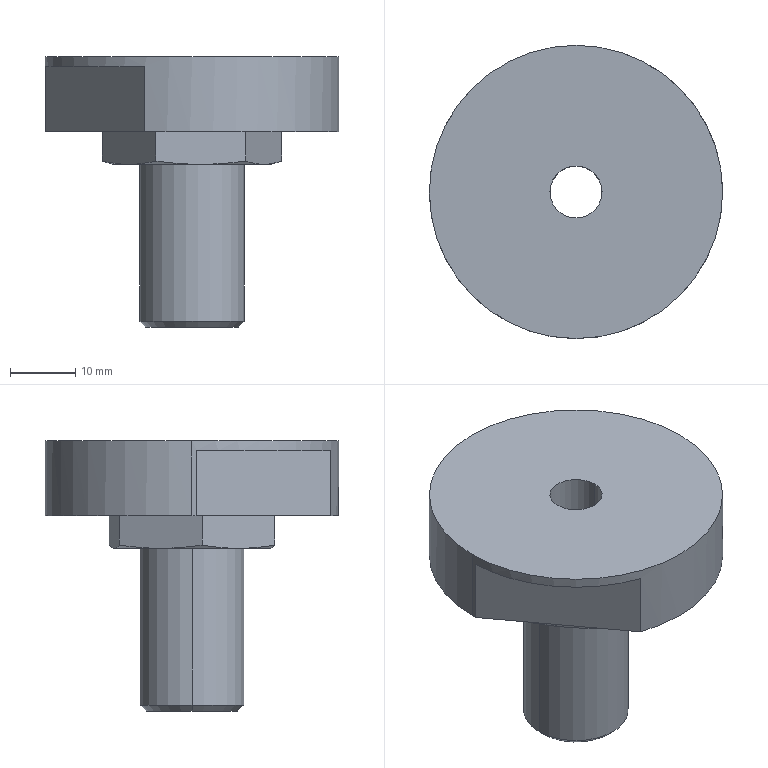Part | SolidWorks | features BaseBody 1 | 1 solid | 34 faces | box 45 x 45 x 41.5 mm | volume 22254 mm3 | plane 14 | cone 12 | cylinder 8 | commonest cylinder face diameters 8 x2 8.566 x2 16 x2 45 x2
STEP:
#1=CARTESIAN_POINT('',(-172.72,21.29,385.481));
#2=VERTEX_POINT('',#1);
#3=CARTESIAN_POINT('',(-202.5,0.,385.481));
#4=VERTEX_POINT('',#3);
#5=CARTESIAN_POINT('',(-180.,0.,385.481));
#6=DIRECTION('',(0.,0.,1.));
#7=DIRECTION('',(1.,0.,0.));
#8=AXIS2_PLACEMENT_3D('',#5,#6,#7);
#9=CIRCLE('',#8,22.5);
#10=EDGE_CURVE('',#2,#4,#9,.T.);
#11=ORIENTED_EDGE('',*,*,#10,.T.);
#12=CARTESIAN_POINT('',(-202.5,0.,396.981));
#13=VERTEX_POINT('',#12);
#14=CARTESIAN_POINT('',(-202.5,0.,391.231));
#15=DIRECTION('',(0.,0.,1.));
#16=VECTOR('',#15,1000.);
#17=LINE('',#14,#16);
#18=EDGE_CURVE('',#4,#13,#17,.T.);
#19=ORIENTED_EDGE('',*,*,#18,.T.);
#20=CARTESIAN_POINT('',(-157.5,0.,396.981));
#21=VERTEX_POINT('',#20);
#22=CARTESIAN_POINT('',(-180.,0.,396.981));
#23=DIRECTION('',(0.,0.,1.));
#24=DIRECTION('',(1.,0.,0.));
#25=AXIS2_PLACEMENT_3D('',#22,#23,#24);
#26=CIRCLE('',#25,22.5);
#27=EDGE_CURVE('',#21,#13,#26,.T.);
#28=ORIENTED_EDGE('',*,*,#27,.F.);
#29=CARTESIAN_POINT('',(-157.5,0.,385.481));
#30=VERTEX_POINT('',#29);
#31=CARTESIAN_POINT('',(-157.5,0.,391.231));
#32=DIRECTION('',(0.,0.,1.));
#33=VECTOR('',#32,1000.);
#34=LINE('',#31,#33);
#35=EDGE_CURVE('',#30,#21,#34,.T.);
#36=ORIENTED_EDGE('',*,*,#35,.F.);
#37=CARTESIAN_POINT('',(-157.51,0.6822,385.481));
#38=VERTEX_POINT('',#37);
#39=CARTESIAN_POINT('',(-180.,0.,385.481));
#40=DIRECTION('',(0.,0.,1.));
#41=DIRECTION('',(1.,0.,0.));
#42=AXIS2_PLACEMENT_3D('',#39,#40,#41);
#43=CIRCLE('',#42,22.5);
#44=EDGE_CURVE('',#30,#38,#43,.T.);
#45=ORIENTED_EDGE('',*,*,#44,.T.);
#46=CARTESIAN_POINT('',(-157.51,0.6822,395.481));
#47=VERTEX_POINT('',#46);
#48=CARTESIAN_POINT('',(-157.51,0.6822,391.231));
#49=DIRECTION('',(0.,0.,1.));
#50=VECTOR('',#49,1000.);
#51=LINE('',#48,#50);
#52=EDGE_CURVE('',#38,#47,#51,.T.);
#53=ORIENTED_EDGE('',*,*,#52,.T.);
#54=CARTESIAN_POINT('',(-172.72,21.29,395.481));
#55=VERTEX_POINT('',#54);
#56=CARTESIAN_POINT('',(-180.,0.,395.481));
#57=DIRECTION('',(0.,0.,1.));
#58=DIRECTION('',(1.,0.,0.));
#59=AXIS2_PLACEMENT_3D('',#56,#57,#58);
#60=CIRCLE('',#59,22.5);
#61=EDGE_CURVE('',#47,#55,#60,.T.);
#62=ORIENTED_EDGE('',*,*,#61,.T.);
#63=CARTESIAN_POINT('',(-172.72,21.29,391.231));
#64=DIRECTION('',(0.,0.,-1.));
#65=VECTOR('',#64,1000.);
#66=LINE('',#63,#65);
#67=EDGE_CURVE('',#55,#2,#66,.T.);
#68=ORIENTED_EDGE('',*,*,#67,.T.);
#69=EDGE_LOOP('',(#11,#19,#28,#36,#45,#53,#62,#68));
#70=FACE_OUTER_BOUND('',#69,.T.);
#71=CARTESIAN_POINT('',(-180.,0.,391.231));
#72=DIRECTION('',(0.,0.,1.));
#73=DIRECTION('',(1.,0.,0.));
#74=AXIS2_PLACEMENT_3D('',#71,#72,#73);
#75=CYLINDRICAL_SURFACE('',#74,22.5);
#76=ADVANCED_FACE('',(#70),#75,.T.);
#77=CARTESIAN_POINT('',(-184.,0.,361.844));
#78=VERTEX_POINT('',#77);
#79=CARTESIAN_POINT('',(-176.,0.,361.844));
#80=VERTEX_POINT('',#79);
#81=CARTESIAN_POINT('',(-180.,0.,361.844));
#82=DIRECTION('',(0.,0.,1.));
#83=DIRECTION('',(1.,0.,0.));
#84=AXIS2_PLACEMENT_3D('',#81,#82,#83);
#85=CIRCLE('',#84,4.);
#86=EDGE_CURVE('',#78,#80,#85,.T.);
#87=ORIENTED_EDGE('',*,*,#86,.F.);
#88=CARTESIAN_POINT('',(-184.,0.,396.981));
#89=VERTEX_POINT('',#88);
#90=CARTESIAN_POINT('',(-184.,0.,379.413));
#91=DIRECTION('',(0.,0.,1.));
#92=VECTOR('',#91,1000.);
#93=LINE('',#90,#92);
#94=EDGE_CURVE('',#78,#89,#93,.T.);
#95=ORIENTED_EDGE('',*,*,#94,.T.);
#96=CARTESIAN_POINT('',(-176.,0.,396.981));
#97=VERTEX_POINT('',#96);
#98=CARTESIAN_POINT('',(-180.,0.,396.981));
#99=DIRECTION('',(0.,0.,-1.));
#100=DIRECTION('',(1.,0.,0.));
#101=AXIS2_PLACEMENT_3D('',#98,#99,#100);
#102=CIRCLE('',#101,4.);
#103=EDGE_CURVE('',#97,#89,#102,.T.);
#104=ORIENTED_EDGE('',*,*,#103,.F.);
#105=CARTESIAN_POINT('',(-176.,0.,379.413));
#106=DIRECTION('',(0.,0.,1.));
#107=VECTOR('',#106,1000.);
#108=LINE('',#105,#107);
#109=EDGE_CURVE('',#80,#97,#108,.T.);
#110=ORIENTED_EDGE('',*,*,#109,.F.);
#111=EDGE_LOOP('',(#87,#95,#104,#110));
#112=FACE_OUTER_BOUND('',#111,.T.);
#113=CARTESIAN_POINT('',(-180.,0.,379.413));
#114=DIRECTION('',(0.,0.,1.));
#115=DIRECTION('',(1.,0.,0.));
#116=AXIS2_PLACEMENT_3D('',#113,#114,#115);
#117=CYLINDRICAL_SURFACE('',#116,4.);
#118=ADVANCED_FACE('',(#112),#117,.F.);
#119=ORIENTED_EDGE('',*,*,#86,.T.);
#120=CARTESIAN_POINT('',(-175.717,0.,361.681));
#121=VERTEX_POINT('',#120);
#122=CARTESIAN_POINT('',(-175.717,0.,361.681));
#123=DIRECTION('',(0.866,0.,-0.5));
#124=VECTOR('',#123,1000.);
#125=LINE('',#122,#124);
#126=EDGE_CURVE('',#80,#121,#125,.T.);
#127=ORIENTED_EDGE('',*,*,#126,.T.);
#128=CARTESIAN_POINT('',(-184.283,0.,361.681));
#129=VERTEX_POINT('',#128);
#130=CARTESIAN_POINT('',(-180.,0.,361.681));
#131=DIRECTION('',(0.,0.,1.));
#132=DIRECTION('',(-0.8046,-0.5938,0.));
#133=AXIS2_PLACEMENT_3D('',#130,#131,#132);
#134=CIRCLE('',#133,4.283);
#135=EDGE_CURVE('',#129,#121,#134,.T.);
#136=ORIENTED_EDGE('',*,*,#135,.F.);
#137=CARTESIAN_POINT('',(-184.283,0.,361.681));
#138=DIRECTION('',(-0.866,0.,-0.5));
#139=VECTOR('',#138,1000.);
#140=LINE('',#137,#139);
#141=EDGE_CURVE('',#78,#129,#140,.T.);
#142=ORIENTED_EDGE('',*,*,#141,.F.);
#143=EDGE_LOOP('',(#119,#127,#136,#142));
#144=FACE_OUTER_BOUND('',#143,.T.);
#145=CARTESIAN_POINT('',(-180.,0.,361.681));
#146=DIRECTION('',(0.,0.,-1.));
#147=DIRECTION('',(-1.,0.,0.));
#148=AXIS2_PLACEMENT_3D('',#145,#146,#147);
#149=CONICAL_SURFACE('',#148,4.283,1.047);
#150=ADVANCED_FACE('',(#144),#149,.F.);
#151=CARTESIAN_POINT('',(-184.283,0.,356.062));
#152=VERTEX_POINT('',#151);
#153=CARTESIAN_POINT('',(-175.717,0.,356.062));
#154=VERTEX_POINT('',#153);
#155=CARTESIAN_POINT('',(-180.,0.,356.062));
#156=DIRECTION('',(0.,0.,1.));
#157=DIRECTION('',(1.,0.,0.));
#158=AXIS2_PLACEMENT_3D('',#155,#156,#157);
#159=CIRCLE('',#158,4.283);
#160=EDGE_CURVE('',#152,#154,#159,.T.);
#161=ORIENTED_EDGE('',*,*,#160,.F.);
#162=CARTESIAN_POINT('',(-184.283,0.,358.872));
#163=DIRECTION('',(0.,0.,1.));
#164=VECTOR('',#163,1000.);
#165=LINE('',#162,#164);
#166=EDGE_CURVE('',#152,#129,#165,.T.);
#167=ORIENTED_EDGE('',*,*,#166,.T.);
#168=ORIENTED_EDGE('',*,*,#135,.T.);
#169=CARTESIAN_POINT('',(-175.717,0.,358.872));
#170=DIRECTION('',(0.,0.,1.));
#171=VECTOR('',#170,1000.);
#172=LINE('',#169,#171);
#173=EDGE_CURVE('',#154,#121,#172,.T.);
#174=ORIENTED_EDGE('',*,*,#173,.F.);
#175=EDGE_LOOP('',(#161,#167,#168,#174));
#176=FACE_OUTER_BOUND('',#175,.T.);
#177=CARTESIAN_POINT('',(-180.,0.,358.872));
#178=DIRECTION('',(0.,0.,1.));
#179=DIRECTION('',(1.,0.,0.));
#180=AXIS2_PLACEMENT_3D('',#177,#178,#179);
#181=CYLINDRICAL_SURFACE('',#180,4.283);
#182=ADVANCED_FACE('',(#176),#181,.F.);
#183=ORIENTED_EDGE('',*,*,#160,.T.);
#184=CARTESIAN_POINT('',(-175.136,0.,355.481));
#185=VERTEX_POINT('',#184);
#186=CARTESIAN_POINT('',(-175.136,0.,355.481));
#187=DIRECTION('',(0.7071,0.,-0.7071));
#188=VECTOR('',#187,1000.);
#189=LINE('',#186,#188);
#190=EDGE_CURVE('',#154,#185,#189,.T.);
#191=ORIENTED_EDGE('',*,*,#190,.T.);
#192=CARTESIAN_POINT('',(-184.864,0.,355.481));
#193=VERTEX_POINT('',#192);
#194=CARTESIAN_POINT('',(-180.,0.,355.481));
#195=DIRECTION('',(0.,0.,1.));
#196=DIRECTION('',(-1.,0.,0.));
#197=AXIS2_PLACEMENT_3D('',#194,#195,#196);
#198=CIRCLE('',#197,4.864);
#199=EDGE_CURVE('',#193,#185,#198,.T.);
#200=ORIENTED_EDGE('',*,*,#199,.F.);
#201=CARTESIAN_POINT('',(-184.864,0.,355.481));
#202=DIRECTION('',(-0.7071,0.,-0.7071));
#203=VECTOR('',#202,1000.);
#204=LINE('',#201,#203);
#205=EDGE_CURVE('',#152,#193,#204,.T.);
#206=ORIENTED_EDGE('',*,*,#205,.F.);
#207=EDGE_LOOP('',(#183,#191,#200,#206));
#208=FACE_OUTER_BOUND('',#207,.T.);
#209=CARTESIAN_POINT('',(-180.,0.,355.481));
#210=DIRECTION('',(0.,0.,-1.));
#211=DIRECTION('',(-1.,0.,0.));
#212=AXIS2_PLACEMENT_3D('',#209,#210,#211);
#213=CONICAL_SURFACE('',#212,4.864,0.7854);
#214=ADVANCED_FACE('',(#208),#213,.F.);
#215=CARTESIAN_POINT('',(-172.,0.,356.401));
#216=VERTEX_POINT('',#215);
#217=CARTESIAN_POINT('',(-188.,0.,356.401));
#218=VERTEX_POINT('',#217);
#219=CARTESIAN_POINT('',(-180.,0.,356.401));
#220=DIRECTION('',(0.,0.,1.));
#221=DIRECTION('',(1.,0.,0.));
#222=AXIS2_PLACEMENT_3D('',#219,#220,#221);
#223=CIRCLE('',#222,8.);
#224=EDGE_CURVE('',#216,#218,#223,.T.);
#225=ORIENTED_EDGE('',*,*,#224,.T.);
#226=CARTESIAN_POINT('',(-188.,0.,380.481));
#227=VERTEX_POINT('',#226);
#228=CARTESIAN_POINT('',(-188.,0.,368.441));
#229=DIRECTION('',(0.,0.,1.));
#230=VECTOR('',#229,1000.);
#231=LINE('',#228,#230);
#232=EDGE_CURVE('',#218,#227,#231,.T.);
#233=ORIENTED_EDGE('',*,*,#232,.T.);
#234=CARTESIAN_POINT('',(-172.,0.,380.481));
#235=VERTEX_POINT('',#234);
#236=CARTESIAN_POINT('',(-180.,0.,380.481));
#237=DIRECTION('',(0.,0.,1.));
#238=DIRECTION('',(1.,0.,0.));
#239=AXIS2_PLACEMENT_3D('',#236,#237,#238);
#240=CIRCLE('',#239,8.);
#241=EDGE_CURVE('',#235,#227,#240,.T.);
#242=ORIENTED_EDGE('',*,*,#241,.F.);
#243=CARTESIAN_POINT('',(-172.,0.,368.441));
#244=DIRECTION('',(0.,0.,1.));
#245=VECTOR('',#244,1000.);
#246=LINE('',#243,#245);
#247=EDGE_CURVE('',#216,#235,#246,.T.);
#248=ORIENTED_EDGE('',*,*,#247,.F.);
#249=EDGE_LOOP('',(#225,#233,#242,#248));
#250=FACE_OUTER_BOUND('',#249,.T.);
#251=CARTESIAN_POINT('',(-180.,0.,368.441));
#252=DIRECTION('',(0.,0.,1.));
#253=DIRECTION('',(1.,0.,0.));
#254=AXIS2_PLACEMENT_3D('',#251,#252,#253);
#255=CYLINDRICAL_SURFACE('',#254,8.);
#256=ADVANCED_FACE('',(#250),#255,.T.);
#257=CARTESIAN_POINT('',(-187.08,0.,355.481));
#258=VERTEX_POINT('',#257);
#259=CARTESIAN_POINT('',(-172.92,0.,355.481));
#260=VERTEX_POINT('',#259);
#261=CARTESIAN_POINT('',(-180.,0.,355.481));
#262=DIRECTION('',(0.,0.,-1.));
#263=DIRECTION('',(1.,0.,0.));
#264=AXIS2_PLACEMENT_3D('',#261,#262,#263);
#265=CIRCLE('',#264,7.08);
#266=EDGE_CURVE('',#258,#260,#265,.T.);
#267=ORIENTED_EDGE('',*,*,#266,.F.);
#268=CARTESIAN_POINT('',(-188.,0.,356.401));
#269=DIRECTION('',(-0.7071,0.,0.7071));
#270=VECTOR('',#269,1000.);
#271=LINE('',#268,#270);
#272=EDGE_CURVE('',#258,#218,#271,.T.);
#273=ORIENTED_EDGE('',*,*,#272,.T.);
#274=ORIENTED_EDGE('',*,*,#224,.F.);
#275=CARTESIAN_POINT('',(-172.,0.,356.401));
#276=DIRECTION('',(0.7071,0.,0.7071));
#277=VECTOR('',#276,1000.);
#278=LINE('',#275,#277);
#279=EDGE_CURVE('',#260,#216,#278,.T.);
#280=ORIENTED_EDGE('',*,*,#279,.F.);
#281=EDGE_LOOP('',(#267,#273,#274,#280));
#282=FACE_OUTER_BOUND('',#281,.T.);
#283=CARTESIAN_POINT('',(-180.,0.,356.401));
#284=DIRECTION('',(0.,0.,1.));
#285=DIRECTION('',(1.,0.,0.));
#286=AXIS2_PLACEMENT_3D('',#283,#284,#285);
#287=CONICAL_SURFACE('',#286,8.,0.7854);
#288=ADVANCED_FACE('',(#282),#287,.T.);
#289=ORIENTED_EDGE('',*,*,#27,.T.);
#290=CARTESIAN_POINT('',(-180.,0.,396.981));
#291=DIRECTION('',(0.,0.,1.));
#292=DIRECTION('',(1.,0.,0.));
#293=AXIS2_PLACEMENT_3D('',#290,#291,#292);
#294=CIRCLE('',#293,22.5);
#295=EDGE_CURVE('',#13,#21,#294,.T.);
#296=ORIENTED_EDGE('',*,*,#295,.T.);
#297=EDGE_LOOP('',(#289,#296));
#298=FACE_OUTER_BOUND('',#297,.T.);
#299=ORIENTED_EDGE('',*,*,#103,.T.);
#300=CARTESIAN_POINT('',(-180.,0.,396.981));
#301=DIRECTION('',(0.,0.,-1.));
#302=DIRECTION('',(1.,0.,0.));
#303=AXIS2_PLACEMENT_3D('',#300,#301,#302);
#304=CIRCLE('',#303,4.);
#305=EDGE_CURVE('',#89,#97,#304,.T.);
#306=ORIENTED_EDGE('',*,*,#305,.T.);
#307=EDGE_LOOP('',(#299,#306));
#308=FACE_BOUND('',#307,.T.);
#309=CARTESIAN_POINT('',(-187.868,10.661,396.981));
#310=DIRECTION('',(0.,0.,1.));
#311=DIRECTION('',(1.,0.,0.));
#312=AXIS2_PLACEMENT_3D('',#309,#310,#311);
#313=PLANE('',#312);
#314=ADVANCED_FACE('',(#298,#308),#313,.T.);
#315=ORIENTED_EDGE('',*,*,#18,.F.);
#316=CARTESIAN_POINT('',(-202.49,-0.6822,385.481));
#317=VERTEX_POINT('',#316);
#318=CARTESIAN_POINT('',(-180.,0.,385.481));
#319=DIRECTION('',(0.,0.,1.));
#320=DIRECTION('',(1.,0.,0.));
#321=AXIS2_PLACEMENT_3D('',#318,#319,#320);
#322=CIRCLE('',#321,22.5);
#323=EDGE_CURVE('',#4,#317,#322,.T.);
#324=ORIENTED_EDGE('',*,*,#323,.T.);
#325=CARTESIAN_POINT('',(-202.49,-0.6822,395.481));
#326=VERTEX_POINT('',#325);
#327=CARTESIAN_POINT('',(-202.49,-0.6822,391.231));
#328=DIRECTION('',(0.,0.,1.));
#329=VECTOR('',#328,1000.);
#330=LINE('',#327,#329);
#331=EDGE_CURVE('',#317,#326,#330,.T.);
#332=ORIENTED_EDGE('',*,*,#331,.T.);
#333=CARTESIAN_POINT('',(-187.28,-21.29,395.481));
#334=VERTEX_POINT('',#333);
#335=CARTESIAN_POINT('',(-180.,0.,395.481));
#336=DIRECTION('',(0.,0.,1.));
#337=DIRECTION('',(1.,0.,0.));
#338=AXIS2_PLACEMENT_3D('',#335,#336,#337);
#339=CIRCLE('',#338,22.5);
#340=EDGE_CURVE('',#326,#334,#339,.T.);
#341=ORIENTED_EDGE('',*,*,#340,.T.);
#342=CARTESIAN_POINT('',(-187.28,-21.29,385.481));
#343=VERTEX_POINT('',#342);
#344=CARTESIAN_POINT('',(-187.28,-21.29,391.231));
#345=DIRECTION('',(0.,0.,-1.));
#346=VECTOR('',#345,1000.);
#347=LINE('',#344,#346);
#348=EDGE_CURVE('',#334,#343,#347,.T.);
#349=ORIENTED_EDGE('',*,*,#348,.T.);
#350=CARTESIAN_POINT('',(-180.,0.,385.481));
#351=DIRECTION('',(0.,0.,1.));
#352=DIRECTION('',(1.,0.,0.));
#353=AXIS2_PLACEMENT_3D('',#350,#351,#352);
#354=CIRCLE('',#353,22.5);
#355=EDGE_CURVE('',#343,#30,#354,.T.);
#356=ORIENTED_EDGE('',*,*,#355,.T.);
#357=ORIENTED_EDGE('',*,*,#35,.T.);
#358=ORIENTED_EDGE('',*,*,#295,.F.);
#359=EDGE_LOOP('',(#315,#324,#332,#341,#349,#356,#357,#358));
#360=FACE_OUTER_BOUND('',#359,.T.);
#361=CARTESIAN_POINT('',(-180.,0.,391.231));
#362=DIRECTION('',(0.,0.,1.));
#363=DIRECTION('',(1.,0.,0.));
#364=AXIS2_PLACEMENT_3D('',#361,#362,#363);
#365=CYLINDRICAL_SURFACE('',#364,22.5);
#366=ADVANCED_FACE('',(#360),#365,.T.);
#367=ORIENTED_EDGE('',*,*,#94,.F.);
#368=CARTESIAN_POINT('',(-180.,0.,361.844));
#369=DIRECTION('',(0.,0.,1.));
#370=DIRECTION('',(1.,0.,0.));
#371=AXIS2_PLACEMENT_3D('',#368,#369,#370);
#372=CIRCLE('',#371,4.);
#373=EDGE_CURVE('',#80,#78,#372,.T.);
#374=ORIENTED_EDGE('',*,*,#373,.F.);
#375=ORIENTED_EDGE('',*,*,#109,.T.);
#376=ORIENTED_EDGE('',*,*,#305,.F.);
#377=EDGE_LOOP('',(#367,#374,#375,#376));
#378=FACE_OUTER_BOUND('',#377,.T.);
#379=CARTESIAN_POINT('',(-180.,0.,379.413));
#380=DIRECTION('',(0.,0.,1.));
#381=DIRECTION('',(1.,0.,0.));
#382=AXIS2_PLACEMENT_3D('',#379,#380,#381);
#383=CYLINDRICAL_SURFACE('',#382,4.);
#384=ADVANCED_FACE('',(#378),#383,.F.);
#385=CARTESIAN_POINT('',(-187.28,-21.29,385.481));
#386=DIRECTION('',(-0.5938,0.8046,0.));
#387=VECTOR('',#386,1000.);
#388=LINE('',#385,#387);
#389=EDGE_CURVE('',#343,#317,#388,.T.);
#390=ORIENTED_EDGE('',*,*,#389,.T.);
#391=ORIENTED_EDGE('',*,*,#323,.F.);
#392=ORIENTED_EDGE('',*,*,#10,.F.);
#393=CARTESIAN_POINT('',(-172.72,21.29,385.481));
#394=DIRECTION('',(0.5938,-0.8046,0.));
#395=VECTOR('',#394,1000.);
#396=LINE('',#393,#395);
#397=EDGE_CURVE('',#2,#38,#396,.T.);
#398=ORIENTED_EDGE('',*,*,#397,.T.);
#399=ORIENTED_EDGE('',*,*,#44,.F.);
#400=ORIENTED_EDGE('',*,*,#355,.F.);
#401=EDGE_LOOP('',(#390,#391,#392,#398,#399,#400));
#402=FACE_OUTER_BOUND('',#401,.T.);
#403=CARTESIAN_POINT('',(-174.459,12.7,385.481));
#404=VERTEX_POINT('',#403);
#405=CARTESIAN_POINT('',(-188.228,11.149,385.481));
#406=VERTEX_POINT('',#405);
#407=CARTESIAN_POINT('',(-174.459,12.7,385.481));
#408=DIRECTION('',(-0.9937,-0.112,0.));
#409=VECTOR('',#408,1000.);
#410=LINE('',#407,#409);
#411=EDGE_CURVE('',#404,#406,#410,.T.);
#412=ORIENTED_EDGE('',*,*,#411,.T.);
#413=CARTESIAN_POINT('',(-193.769,-1.552,385.481));
#414=VERTEX_POINT('',#413);
#415=CARTESIAN_POINT('',(-188.228,11.149,385.481));
#416=DIRECTION('',(-0.3999,-0.9166,0.));
#417=VECTOR('',#416,1000.);
#418=LINE('',#415,#417);
#419=EDGE_CURVE('',#406,#414,#418,.T.);
#420=ORIENTED_EDGE('',*,*,#419,.T.);
#421=CARTESIAN_POINT('',(-185.541,-12.7,385.481));
#422=VERTEX_POINT('',#421);
#423=CARTESIAN_POINT('',(-193.769,-1.552,385.481));
#424=DIRECTION('',(0.5938,-0.8046,0.));
#425=VECTOR('',#424,1000.);
#426=LINE('',#423,#425);
#427=EDGE_CURVE('',#414,#422,#426,.T.);
#428=ORIENTED_EDGE('',*,*,#427,.T.);
#429=CARTESIAN_POINT('',(-171.772,-11.149,385.481));
#430=VERTEX_POINT('',#429);
#431=CARTESIAN_POINT('',(-185.541,-12.7,385.481));
#432=DIRECTION('',(0.9937,0.112,0.));
#433=VECTOR('',#432,1000.);
#434=LINE('',#431,#433);
#435=EDGE_CURVE('',#422,#430,#434,.T.);
#436=ORIENTED_EDGE('',*,*,#435,.T.);
#437=CARTESIAN_POINT('',(-166.231,1.552,385.481));
#438=VERTEX_POINT('',#437);
#439=CARTESIAN_POINT('',(-171.772,-11.149,385.481));
#440=DIRECTION('',(0.3999,0.9166,0.));
#441=VECTOR('',#440,1000.);
#442=LINE('',#439,#441);
#443=EDGE_CURVE('',#430,#438,#442,.T.);
#444=ORIENTED_EDGE('',*,*,#443,.T.);
#445=CARTESIAN_POINT('',(-166.231,1.552,385.481));
#446=DIRECTION('',(-0.5938,0.8046,0.));
#447=VECTOR('',#446,1000.);
#448=LINE('',#445,#447);
#449=EDGE_CURVE('',#438,#404,#448,.T.);
#450=ORIENTED_EDGE('',*,*,#449,.T.);
#451=EDGE_LOOP('',(#412,#420,#428,#436,#444,#450));
#452=FACE_BOUND('',#451,.T.);
#453=CARTESIAN_POINT('',(-192.381,16.776,385.481));
#454=DIRECTION('',(0.,0.,-1.));
#455=DIRECTION('',(-1.,0.,0.));
#456=AXIS2_PLACEMENT_3D('',#453,#454,#455);
#457=PLANE('',#456);
#458=ADVANCED_FACE('',(#402,#452),#457,.T.);
#459=ORIENTED_EDGE('',*,*,#67,.F.);
#460=CARTESIAN_POINT('',(-188.869,43.169,395.481));
#461=DIRECTION('',(-0.5938,0.8046,0.));
#462=VECTOR('',#461,1000.);
#463=LINE('',#460,#462);
#464=EDGE_CURVE('',#47,#55,#463,.T.);
#465=ORIENTED_EDGE('',*,*,#464,.F.);
#466=ORIENTED_EDGE('',*,*,#52,.F.);
#467=ORIENTED_EDGE('',*,*,#397,.F.);
#468=EDGE_LOOP('',(#459,#465,#466,#467));
#469=FACE_OUTER_BOUND('',#468,.T.);
#470=CARTESIAN_POINT('',(-188.869,43.169,395.481));
#471=DIRECTION('',(-0.8046,-0.5938,0.));
#472=DIRECTION('',(0.5938,-0.8046,0.));
#473=AXIS2_PLACEMENT_3D('',#470,#471,#472);
#474=PLANE('',#473);
#475=ADVANCED_FACE('',(#469),#474,.F.);
#476=ORIENTED_EDGE('',*,*,#61,.F.);
#477=ORIENTED_EDGE('',*,*,#464,.T.);
#478=EDGE_LOOP('',(#476,#477));
#479=FACE_OUTER_BOUND('',#478,.T.);
#480=CARTESIAN_POINT('',(-180.,0.,395.481));
#481=DIRECTION('',(0.,0.,-1.));
#482=DIRECTION('',(-1.,0.,0.));
#483=AXIS2_PLACEMENT_3D('',#480,#481,#482);
#484=PLANE('',#483);
#485=ADVANCED_FACE('',(#479),#484,.T.);
#486=ORIENTED_EDGE('',*,*,#348,.F.);
#487=CARTESIAN_POINT('',(-171.131,-43.169,395.481));
#488=DIRECTION('',(0.5938,-0.8046,0.));
#489=VECTOR('',#488,1000.);
#490=LINE('',#487,#489);
#491=EDGE_CURVE('',#326,#334,#490,.T.);
#492=ORIENTED_EDGE('',*,*,#491,.F.);
#493=ORIENTED_EDGE('',*,*,#331,.F.);
#494=ORIENTED_EDGE('',*,*,#389,.F.);
#495=EDGE_LOOP('',(#486,#492,#493,#494));
#496=FACE_OUTER_BOUND('',#495,.T.);
#497=CARTESIAN_POINT('',(-171.131,-43.169,395.481));
#498=DIRECTION('',(0.8046,0.5938,0.));
#499=DIRECTION('',(-0.5938,0.8046,0.));
#500=AXIS2_PLACEMENT_3D('',#497,#498,#499);
#501=PLANE('',#500);
#502=ADVANCED_FACE('',(#496),#501,.F.);
#503=ORIENTED_EDGE('',*,*,#340,.F.);
#504=ORIENTED_EDGE('',*,*,#491,.T.);
#505=EDGE_LOOP('',(#503,#504));
#506=FACE_OUTER_BOUND('',#505,.T.);
#507=CARTESIAN_POINT('',(-180.,0.,395.481));
#508=DIRECTION('',(0.,0.,-1.));
#509=DIRECTION('',(-1.,0.,0.));
#510=AXIS2_PLACEMENT_3D('',#507,#508,#509);
#511=PLANE('',#510);
#512=ADVANCED_FACE('',(#506),#511,.T.);
#513=ORIENTED_EDGE('',*,*,#126,.F.);
#514=ORIENTED_EDGE('',*,*,#373,.T.);
#515=ORIENTED_EDGE('',*,*,#141,.T.);
#516=CARTESIAN_POINT('',(-180.,0.,361.681));
#517=DIRECTION('',(0.,0.,1.));
#518=DIRECTION('',(-0.8046,-0.5938,0.));
#519=AXIS2_PLACEMENT_3D('',#516,#517,#518);
#520=CIRCLE('',#519,4.283);
#521=EDGE_CURVE('',#121,#129,#520,.T.);
#522=ORIENTED_EDGE('',*,*,#521,.F.);
#523=EDGE_LOOP('',(#513,#514,#515,#522));
#524=FACE_OUTER_BOUND('',#523,.T.);
#525=CARTESIAN_POINT('',(-180.,0.,361.681));
#526=DIRECTION('',(0.,0.,-1.));
#527=DIRECTION('',(-1.,0.,0.));
#528=AXIS2_PLACEMENT_3D('',#525,#526,#527);
#529=CONICAL_SURFACE('',#528,4.283,1.047);
#530=ADVANCED_FACE('',(#524),#529,.F.);
#531=CARTESIAN_POINT('',(-193.769,-1.552,380.978));
#532=VERTEX_POINT('',#531);
#533=CARTESIAN_POINT('',(-193.769,-1.552,385.481));
#534=DIRECTION('',(0.,0.,-1.));
#535=VECTOR('',#534,1000.);
#536=LINE('',#533,#535);
#537=EDGE_CURVE('',#414,#532,#536,.T.);
#538=ORIENTED_EDGE('',*,*,#537,.F.);
#539=ORIENTED_EDGE('',*,*,#419,.F.);
#540=CARTESIAN_POINT('',(-188.228,11.149,380.978));
#541=VERTEX_POINT('',#540);
#542=CARTESIAN_POINT('',(-188.228,11.149,385.481));
#543=DIRECTION('',(0.,0.,1.));
#544=VECTOR('',#543,1000.);
#545=LINE('',#542,#544);
#546=EDGE_CURVE('',#541,#406,#545,.T.);
#547=ORIENTED_EDGE('',*,*,#546,.F.);
#548=CARTESIAN_POINT('',(-190.999,4.798,380.481));
#549=VERTEX_POINT('',#548);
#550=CARTESIAN_POINT('',(-190.999,4.798,380.481));
#551=CARTESIAN_POINT('',(-190.535,5.862,380.481));
#552=CARTESIAN_POINT('',(-190.072,6.923,380.527));
#553=CARTESIAN_POINT('',(-189.149,9.039,380.699));
#554=CARTESIAN_POINT('',(-188.688,10.095,380.824));
#555=CARTESIAN_POINT('',(-188.228,11.149,380.978));
#556=B_SPLINE_CURVE_WITH_KNOTS('',3,(#550,#551,#552,#553,#554,#555),.UNSPECIFIED.,.F.,.F.,(4,2,4),(0.,0.003473,0.006946),.UNSPECIFIED.);
#557=EDGE_CURVE('',#549,#541,#556,.T.);
#558=ORIENTED_EDGE('',*,*,#557,.F.);
#559=CARTESIAN_POINT('',(-193.769,-1.552,380.978));
#560=CARTESIAN_POINT('',(-193.31,-0.498,380.824));
#561=CARTESIAN_POINT('',(-192.849,0.5576,380.699));
#562=CARTESIAN_POINT('',(-191.926,2.674,380.527));
#563=CARTESIAN_POINT('',(-191.463,3.735,380.481));
#564=CARTESIAN_POINT('',(-190.999,4.798,380.481));
#565=B_SPLINE_CURVE_WITH_KNOTS('',3,(#559,#560,#561,#562,#563,#564),.UNSPECIFIED.,.F.,.F.,(4,2,4),(0.,0.003473,0.006946),.UNSPECIFIED.);
#566=EDGE_CURVE('',#532,#549,#565,.T.);
#567=ORIENTED_EDGE('',*,*,#566,.F.);
#568=EDGE_LOOP('',(#538,#539,#547,#558,#567));
#569=FACE_OUTER_BOUND('',#568,.T.);
#570=CARTESIAN_POINT('',(-193.769,-1.552,385.481));
#571=DIRECTION('',(0.9166,-0.3999,0.));
#572=DIRECTION('',(0.3999,0.9166,0.));
#573=AXIS2_PLACEMENT_3D('',#570,#571,#572);
#574=PLANE('',#573);
#575=ADVANCED_FACE('',(#569),#574,.F.);
#576=ORIENTED_EDGE('',*,*,#411,.F.);
#577=CARTESIAN_POINT('',(-174.459,12.7,380.978));
#578=VERTEX_POINT('',#577);
#579=CARTESIAN_POINT('',(-174.459,12.7,385.481));
#580=DIRECTION('',(0.,0.,1.));
#581=VECTOR('',#580,1000.);
#582=LINE('',#579,#581);
#583=EDGE_CURVE('',#578,#404,#582,.T.);
#584=ORIENTED_EDGE('',*,*,#583,.F.);
#585=CARTESIAN_POINT('',(-181.344,11.925,380.481));
#586=VERTEX_POINT('',#585);
#587=CARTESIAN_POINT('',(-181.344,11.925,380.481));
#588=CARTESIAN_POINT('',(-180.19,12.054,380.481));
#589=CARTESIAN_POINT('',(-179.04,12.184,380.527));
#590=CARTESIAN_POINT('',(-176.746,12.443,380.699));
#591=CARTESIAN_POINT('',(-175.602,12.572,380.824));
#592=CARTESIAN_POINT('',(-174.459,12.7,380.978));
#593=B_SPLINE_CURVE_WITH_KNOTS('',3,(#587,#588,#589,#590,#591,#592),.UNSPECIFIED.,.F.,.F.,(4,2,4),(0.,0.003473,0.006946),.UNSPECIFIED.);
#594=EDGE_CURVE('',#586,#578,#593,.T.);
#595=ORIENTED_EDGE('',*,*,#594,.F.);
#596=CARTESIAN_POINT('',(-188.228,11.149,380.978));
#597=CARTESIAN_POINT('',(-187.086,11.277,380.824));
#598=CARTESIAN_POINT('',(-185.942,11.406,380.699));
#599=CARTESIAN_POINT('',(-183.647,11.665,380.527));
#600=CARTESIAN_POINT('',(-182.497,11.795,380.481));
#601=CARTESIAN_POINT('',(-181.344,11.925,380.481));
#602=B_SPLINE_CURVE_WITH_KNOTS('',3,(#596,#597,#598,#599,#600,#601),.UNSPECIFIED.,.F.,.F.,(4,2,4),(0.,0.003473,0.006946),.UNSPECIFIED.);
#603=EDGE_CURVE('',#541,#586,#602,.T.);
#604=ORIENTED_EDGE('',*,*,#603,.F.);
#605=ORIENTED_EDGE('',*,*,#546,.T.);
#606=EDGE_LOOP('',(#576,#584,#595,#604,#605));
#607=FACE_OUTER_BOUND('',#606,.T.);
#608=CARTESIAN_POINT('',(-188.228,11.149,385.481));
#609=DIRECTION('',(0.112,-0.9937,0.));
#610=DIRECTION('',(0.9937,0.112,0.));
#611=AXIS2_PLACEMENT_3D('',#608,#609,#610);
#612=PLANE('',#611);
#613=ADVANCED_FACE('',(#607),#612,.F.);
#614=ORIENTED_EDGE('',*,*,#449,.F.);
#615=CARTESIAN_POINT('',(-166.231,1.552,380.978));
#616=VERTEX_POINT('',#615);
#617=CARTESIAN_POINT('',(-166.231,1.552,385.481));
#618=DIRECTION('',(0.,0.,1.));
#619=VECTOR('',#618,1000.);
#620=LINE('',#617,#619);
#621=EDGE_CURVE('',#616,#438,#620,.T.);
#622=ORIENTED_EDGE('',*,*,#621,.F.);
#623=CARTESIAN_POINT('',(-170.345,7.126,380.481));
#624=VERTEX_POINT('',#623);
#625=CARTESIAN_POINT('',(-170.345,7.126,380.481));
#626=CARTESIAN_POINT('',(-169.656,6.192,380.481));
#627=CARTESIAN_POINT('',(-168.968,5.261,380.527));
#628=CARTESIAN_POINT('',(-167.597,3.403,380.699));
#629=CARTESIAN_POINT('',(-166.913,2.477,380.824));
#630=CARTESIAN_POINT('',(-166.231,1.552,380.978));
#631=B_SPLINE_CURVE_WITH_KNOTS('',3,(#625,#626,#627,#628,#629,#630),.UNSPECIFIED.,.F.,.F.,(4,2,4),(0.,0.003473,0.006946),.UNSPECIFIED.);
#632=EDGE_CURVE('',#624,#616,#631,.T.);
#633=ORIENTED_EDGE('',*,*,#632,.F.);
#634=CARTESIAN_POINT('',(-174.459,12.7,380.978));
#635=CARTESIAN_POINT('',(-173.777,11.775,380.824));
#636=CARTESIAN_POINT('',(-173.093,10.849,380.699));
#637=CARTESIAN_POINT('',(-171.721,8.991,380.527));
#638=CARTESIAN_POINT('',(-171.034,8.06,380.481));
#639=CARTESIAN_POINT('',(-170.345,7.126,380.481));
#640=B_SPLINE_CURVE_WITH_KNOTS('',3,(#634,#635,#636,#637,#638,#639),.UNSPECIFIED.,.F.,.F.,(4,2,4),(0.,0.003473,0.006946),.UNSPECIFIED.);
#641=EDGE_CURVE('',#578,#624,#640,.T.);
#642=ORIENTED_EDGE('',*,*,#641,.F.);
#643=ORIENTED_EDGE('',*,*,#583,.T.);
#644=EDGE_LOOP('',(#614,#622,#633,#642,#643));
#645=FACE_OUTER_BOUND('',#644,.T.);
#646=CARTESIAN_POINT('',(-174.459,12.7,385.481));
#647=DIRECTION('',(-0.8046,-0.5938,0.));
#648=DIRECTION('',(0.5938,-0.8046,0.));
#649=AXIS2_PLACEMENT_3D('',#646,#647,#648);
#650=PLANE('',#649);
#651=ADVANCED_FACE('',(#645),#650,.F.);
#652=ORIENTED_EDGE('',*,*,#443,.F.);
#653=CARTESIAN_POINT('',(-171.772,-11.149,380.978));
#654=VERTEX_POINT('',#653);
#655=CARTESIAN_POINT('',(-171.772,-11.149,385.481));
#656=DIRECTION('',(0.,0.,1.));
#657=VECTOR('',#656,1000.);
#658=LINE('',#655,#657);
#659=EDGE_CURVE('',#654,#430,#658,.T.);
#660=ORIENTED_EDGE('',*,*,#659,.F.);
#661=CARTESIAN_POINT('',(-169.001,-4.798,380.481));
#662=VERTEX_POINT('',#661);
#663=CARTESIAN_POINT('',(-169.001,-4.798,380.481));
#664=CARTESIAN_POINT('',(-169.465,-5.862,380.481));
#665=CARTESIAN_POINT('',(-169.928,-6.923,380.527));
#666=CARTESIAN_POINT('',(-170.851,-9.039,380.699));
#667=CARTESIAN_POINT('',(-171.312,-10.095,380.824));
#668=CARTESIAN_POINT('',(-171.772,-11.149,380.978));
#669=B_SPLINE_CURVE_WITH_KNOTS('',3,(#663,#664,#665,#666,#667,#668),.UNSPECIFIED.,.F.,.F.,(4,2,4),(0.,0.003473,0.006946),.UNSPECIFIED.);
#670=EDGE_CURVE('',#662,#654,#669,.T.);
#671=ORIENTED_EDGE('',*,*,#670,.F.);
#672=CARTESIAN_POINT('',(-166.231,1.552,380.978));
#673=CARTESIAN_POINT('',(-166.69,0.498,380.824));
#674=CARTESIAN_POINT('',(-167.151,-0.5576,380.699));
#675=CARTESIAN_POINT('',(-168.074,-2.674,380.527));
#676=CARTESIAN_POINT('',(-168.537,-3.735,380.481));
#677=CARTESIAN_POINT('',(-169.001,-4.798,380.481));
#678=B_SPLINE_CURVE_WITH_KNOTS('',3,(#672,#673,#674,#675,#676,#677),.UNSPECIFIED.,.F.,.F.,(4,2,4),(0.,0.003473,0.006946),.UNSPECIFIED.);
#679=EDGE_CURVE('',#616,#662,#678,.T.);
#680=ORIENTED_EDGE('',*,*,#679,.F.);
#681=ORIENTED_EDGE('',*,*,#621,.T.);
#682=EDGE_LOOP('',(#652,#660,#671,#680,#681));
#683=FACE_OUTER_BOUND('',#682,.T.);
#684=CARTESIAN_POINT('',(-166.231,1.552,385.481));
#685=DIRECTION('',(-0.9166,0.3999,0.));
#686=DIRECTION('',(-0.3999,-0.9166,0.));
#687=AXIS2_PLACEMENT_3D('',#684,#685,#686);
#688=PLANE('',#687);
#689=ADVANCED_FACE('',(#683),#688,.F.);
#690=ORIENTED_EDGE('',*,*,#659,.T.);
#691=ORIENTED_EDGE('',*,*,#435,.F.);
#692=CARTESIAN_POINT('',(-185.541,-12.7,380.978));
#693=VERTEX_POINT('',#692);
#694=CARTESIAN_POINT('',(-185.541,-12.7,385.481));
#695=DIRECTION('',(0.,0.,1.));
#696=VECTOR('',#695,1000.);
#697=LINE('',#694,#696);
#698=EDGE_CURVE('',#693,#422,#697,.T.);
#699=ORIENTED_EDGE('',*,*,#698,.F.);
#700=CARTESIAN_POINT('',(-178.656,-11.925,380.481));
#701=VERTEX_POINT('',#700);
#702=CARTESIAN_POINT('',(-178.656,-11.925,380.481));
#703=CARTESIAN_POINT('',(-179.81,-12.054,380.481));
#704=CARTESIAN_POINT('',(-180.96,-12.184,380.527));
#705=CARTESIAN_POINT('',(-183.254,-12.443,380.699));
#706=CARTESIAN_POINT('',(-184.398,-12.572,380.824));
#707=CARTESIAN_POINT('',(-185.541,-12.7,380.978));
#708=B_SPLINE_CURVE_WITH_KNOTS('',3,(#702,#703,#704,#705,#706,#707),.UNSPECIFIED.,.F.,.F.,(4,2,4),(0.,0.003473,0.006946),.UNSPECIFIED.);
#709=EDGE_CURVE('',#701,#693,#708,.T.);
#710=ORIENTED_EDGE('',*,*,#709,.F.);
#711=CARTESIAN_POINT('',(-171.772,-11.149,380.978));
#712=CARTESIAN_POINT('',(-172.914,-11.277,380.824));
#713=CARTESIAN_POINT('',(-174.058,-11.406,380.699));
#714=CARTESIAN_POINT('',(-176.353,-11.665,380.527));
#715=CARTESIAN_POINT('',(-177.503,-11.795,380.481));
#716=CARTESIAN_POINT('',(-178.656,-11.925,380.481));
#717=B_SPLINE_CURVE_WITH_KNOTS('',3,(#711,#712,#713,#714,#715,#716),.UNSPECIFIED.,.F.,.F.,(4,2,4),(0.,0.003473,0.006946),.UNSPECIFIED.);
#718=EDGE_CURVE('',#654,#701,#717,.T.);
#719=ORIENTED_EDGE('',*,*,#718,.F.);
#720=EDGE_LOOP('',(#690,#691,#699,#710,#719));
#721=FACE_OUTER_BOUND('',#720,.T.);
#722=CARTESIAN_POINT('',(-171.772,-11.149,385.481));
#723=DIRECTION('',(-0.112,0.9937,0.));
#724=DIRECTION('',(-0.9937,-0.112,0.));
#725=AXIS2_PLACEMENT_3D('',#722,#723,#724);
#726=PLANE('',#725);
#727=ADVANCED_FACE('',(#721),#726,.F.);
#728=ORIENTED_EDGE('',*,*,#698,.T.);
#729=ORIENTED_EDGE('',*,*,#427,.F.);
#730=ORIENTED_EDGE('',*,*,#537,.T.);
#731=CARTESIAN_POINT('',(-189.655,-7.126,380.481));
#732=VERTEX_POINT('',#731);
#733=CARTESIAN_POINT('',(-189.655,-7.126,380.481));
#734=CARTESIAN_POINT('',(-190.344,-6.192,380.481));
#735=CARTESIAN_POINT('',(-191.032,-5.261,380.527));
#736=CARTESIAN_POINT('',(-192.403,-3.403,380.699));
#737=CARTESIAN_POINT('',(-193.087,-2.477,380.824));
#738=CARTESIAN_POINT('',(-193.769,-1.552,380.978));
#739=B_SPLINE_CURVE_WITH_KNOTS('',3,(#733,#734,#735,#736,#737,#738),.UNSPECIFIED.,.F.,.F.,(4,2,4),(0.,0.003473,0.006946),.UNSPECIFIED.);
#740=EDGE_CURVE('',#732,#532,#739,.T.);
#741=ORIENTED_EDGE('',*,*,#740,.F.);
#742=CARTESIAN_POINT('',(-185.541,-12.7,380.978));
#743=CARTESIAN_POINT('',(-186.223,-11.775,380.824));
#744=CARTESIAN_POINT('',(-186.907,-10.849,380.699));
#745=CARTESIAN_POINT('',(-188.279,-8.991,380.527));
#746=CARTESIAN_POINT('',(-188.966,-8.06,380.481));
#747=CARTESIAN_POINT('',(-189.655,-7.126,380.481));
#748=B_SPLINE_CURVE_WITH_KNOTS('',3,(#742,#743,#744,#745,#746,#747),.UNSPECIFIED.,.F.,.F.,(4,2,4),(0.,0.003473,0.006946),.UNSPECIFIED.);
#749=EDGE_CURVE('',#693,#732,#748,.T.);
#750=ORIENTED_EDGE('',*,*,#749,.F.);
#751=EDGE_LOOP('',(#728,#729,#730,#741,#750));
#752=FACE_OUTER_BOUND('',#751,.T.);
#753=CARTESIAN_POINT('',(-185.541,-12.7,385.481));
#754=DIRECTION('',(0.8046,0.5938,0.));
#755=DIRECTION('',(-0.5938,0.8046,0.));
#756=AXIS2_PLACEMENT_3D('',#753,#754,#755);
#757=PLANE('',#756);
#758=ADVANCED_FACE('',(#752),#757,.F.);
#759=ORIENTED_EDGE('',*,*,#166,.F.);
#760=CARTESIAN_POINT('',(-180.,0.,356.062));
#761=DIRECTION('',(0.,0.,1.));
#762=DIRECTION('',(1.,0.,0.));
#763=AXIS2_PLACEMENT_3D('',#760,#761,#762);
#764=CIRCLE('',#763,4.283);
#765=EDGE_CURVE('',#154,#152,#764,.T.);
#766=ORIENTED_EDGE('',*,*,#765,.F.);
#767=ORIENTED_EDGE('',*,*,#173,.T.);
#768=ORIENTED_EDGE('',*,*,#521,.T.);
#769=EDGE_LOOP('',(#759,#766,#767,#768));
#770=FACE_OUTER_BOUND('',#769,.T.);
#771=CARTESIAN_POINT('',(-180.,0.,358.872));
#772=DIRECTION('',(0.,0.,1.));
#773=DIRECTION('',(1.,0.,0.));
#774=AXIS2_PLACEMENT_3D('',#771,#772,#773);
#775=CYLINDRICAL_SURFACE('',#774,4.283);
#776=ADVANCED_FACE('',(#770),#775,.F.);
#777=ORIENTED_EDGE('',*,*,#740,.T.);
#778=ORIENTED_EDGE('',*,*,#566,.T.);
#779=CARTESIAN_POINT('',(-180.,0.,380.481));
#780=DIRECTION('',(0.,0.,1.));
#781=DIRECTION('',(0.,-1.,0.));
#782=AXIS2_PLACEMENT_3D('',#779,#780,#781);
#783=CIRCLE('',#782,12.);
#784=EDGE_CURVE('',#549,#732,#783,.T.);
#785=ORIENTED_EDGE('',*,*,#784,.T.);
#786=EDGE_LOOP('',(#777,#778,#785));
#787=FACE_OUTER_BOUND('',#786,.T.);
#788=CARTESIAN_POINT('',(-180.,0.,380.981));
#789=DIRECTION('',(0.,0.,1.));
#790=DIRECTION('',(0.,-1.,0.));
#791=AXIS2_PLACEMENT_3D('',#788,#789,#790);
#792=CONICAL_SURFACE('',#791,13.868,1.309);
#793=ADVANCED_FACE('',(#787),#792,.T.);
#794=ORIENTED_EDGE('',*,*,#557,.T.);
#795=ORIENTED_EDGE('',*,*,#603,.T.);
#796=CARTESIAN_POINT('',(-180.,0.,380.481));
#797=DIRECTION('',(0.,0.,1.));
#798=DIRECTION('',(1.,0.,0.));
#799=AXIS2_PLACEMENT_3D('',#796,#797,#798);
#800=CIRCLE('',#799,12.);
#801=EDGE_CURVE('',#586,#549,#800,.T.);
#802=ORIENTED_EDGE('',*,*,#801,.T.);
#803=EDGE_LOOP('',(#794,#795,#802));
#804=FACE_OUTER_BOUND('',#803,.T.);
#805=CARTESIAN_POINT('',(-180.,0.,380.981));
#806=DIRECTION('',(0.,0.,1.));
#807=DIRECTION('',(1.,0.,0.));
#808=AXIS2_PLACEMENT_3D('',#805,#806,#807);
#809=CONICAL_SURFACE('',#808,13.868,1.309);
#810=ADVANCED_FACE('',(#804),#809,.T.);
#811=CARTESIAN_POINT('',(-180.,0.,380.481));
#812=DIRECTION('',(0.,0.,1.));
#813=DIRECTION('',(1.,0.,0.));
#814=AXIS2_PLACEMENT_3D('',#811,#812,#813);
#815=CIRCLE('',#814,12.);
#816=EDGE_CURVE('',#624,#586,#815,.T.);
#817=ORIENTED_EDGE('',*,*,#816,.T.);
#818=ORIENTED_EDGE('',*,*,#594,.T.);
#819=ORIENTED_EDGE('',*,*,#641,.T.);
#820=EDGE_LOOP('',(#817,#818,#819));
#821=FACE_OUTER_BOUND('',#820,.T.);
#822=CARTESIAN_POINT('',(-180.,0.,380.981));
#823=DIRECTION('',(0.,0.,1.));
#824=DIRECTION('',(1.,0.,0.));
#825=AXIS2_PLACEMENT_3D('',#822,#823,#824);
#826=CONICAL_SURFACE('',#825,13.868,1.309);
#827=ADVANCED_FACE('',(#821),#826,.T.);
#828=CARTESIAN_POINT('',(-180.,0.,380.481));
#829=DIRECTION('',(0.,0.,1.));
#830=DIRECTION('',(0.,-1.,0.));
#831=AXIS2_PLACEMENT_3D('',#828,#829,#830);
#832=CIRCLE('',#831,12.);
#833=EDGE_CURVE('',#662,#624,#832,.T.);
#834=ORIENTED_EDGE('',*,*,#833,.T.);
#835=ORIENTED_EDGE('',*,*,#632,.T.);
#836=ORIENTED_EDGE('',*,*,#679,.T.);
#837=EDGE_LOOP('',(#834,#835,#836));
#838=FACE_OUTER_BOUND('',#837,.T.);
#839=CARTESIAN_POINT('',(-180.,0.,380.981));
#840=DIRECTION('',(0.,0.,1.));
#841=DIRECTION('',(0.,-1.,0.));
#842=AXIS2_PLACEMENT_3D('',#839,#840,#841);
#843=CONICAL_SURFACE('',#842,13.868,1.309);
#844=ADVANCED_FACE('',(#838),#843,.T.);
#845=CARTESIAN_POINT('',(-180.,0.,380.481));
#846=DIRECTION('',(0.,0.,1.));
#847=DIRECTION('',(1.,0.,0.));
#848=AXIS2_PLACEMENT_3D('',#845,#846,#847);
#849=CIRCLE('',#848,12.);
#850=EDGE_CURVE('',#701,#662,#849,.T.);
#851=ORIENTED_EDGE('',*,*,#850,.T.);
#852=ORIENTED_EDGE('',*,*,#670,.T.);
#853=ORIENTED_EDGE('',*,*,#718,.T.);
#854=EDGE_LOOP('',(#851,#852,#853));
#855=FACE_OUTER_BOUND('',#854,.T.);
#856=CARTESIAN_POINT('',(-180.,0.,380.981));
#857=DIRECTION('',(0.,0.,1.));
#858=DIRECTION('',(1.,0.,0.));
#859=AXIS2_PLACEMENT_3D('',#856,#857,#858);
#860=CONICAL_SURFACE('',#859,13.868,1.309);
#861=ADVANCED_FACE('',(#855),#860,.T.);
#862=ORIENTED_EDGE('',*,*,#709,.T.);
#863=ORIENTED_EDGE('',*,*,#749,.T.);
#864=CARTESIAN_POINT('',(-180.,0.,380.481));
#865=DIRECTION('',(0.,0.,1.));
#866=DIRECTION('',(1.,0.,0.));
#867=AXIS2_PLACEMENT_3D('',#864,#865,#866);
#868=CIRCLE('',#867,12.);
#869=EDGE_CURVE('',#732,#701,#868,.T.);
#870=ORIENTED_EDGE('',*,*,#869,.T.);
#871=EDGE_LOOP('',(#862,#863,#870));
#872=FACE_OUTER_BOUND('',#871,.T.);
#873=CARTESIAN_POINT('',(-180.,0.,380.981));
#874=DIRECTION('',(0.,0.,1.));
#875=DIRECTION('',(1.,0.,0.));
#876=AXIS2_PLACEMENT_3D('',#873,#874,#875);
#877=CONICAL_SURFACE('',#876,13.868,1.309);
#878=ADVANCED_FACE('',(#872),#877,.T.);
#879=ORIENTED_EDGE('',*,*,#190,.F.);
#880=ORIENTED_EDGE('',*,*,#765,.T.);
#881=ORIENTED_EDGE('',*,*,#205,.T.);
#882=CARTESIAN_POINT('',(-180.,0.,355.481));
#883=DIRECTION('',(0.,0.,1.));
#884=DIRECTION('',(-1.,0.,0.));
#885=AXIS2_PLACEMENT_3D('',#882,#883,#884);
#886=CIRCLE('',#885,4.864);
#887=EDGE_CURVE('',#185,#193,#886,.T.);
#888=ORIENTED_EDGE('',*,*,#887,.F.);
#889=EDGE_LOOP('',(#879,#880,#881,#888));
#890=FACE_OUTER_BOUND('',#889,.T.);
#891=CARTESIAN_POINT('',(-180.,0.,355.481));
#892=DIRECTION('',(0.,0.,-1.));
#893=DIRECTION('',(-1.,0.,0.));
#894=AXIS2_PLACEMENT_3D('',#891,#892,#893);
#895=CONICAL_SURFACE('',#894,4.864,0.7854);
#896=ADVANCED_FACE('',(#890),#895,.F.);
#897=ORIENTED_EDGE('',*,*,#241,.T.);
#898=CARTESIAN_POINT('',(-180.,0.,380.481));
#899=DIRECTION('',(0.,0.,1.));
#900=DIRECTION('',(1.,0.,0.));
#901=AXIS2_PLACEMENT_3D('',#898,#899,#900);
#902=CIRCLE('',#901,8.);
#903=EDGE_CURVE('',#227,#235,#902,.T.);
#904=ORIENTED_EDGE('',*,*,#903,.T.);
#905=EDGE_LOOP('',(#897,#904));
#906=FACE_BOUND('',#905,.T.);
#907=ORIENTED_EDGE('',*,*,#833,.F.);
#908=ORIENTED_EDGE('',*,*,#850,.F.);
#909=ORIENTED_EDGE('',*,*,#869,.F.);
#910=ORIENTED_EDGE('',*,*,#784,.F.);
#911=ORIENTED_EDGE('',*,*,#801,.F.);
#912=ORIENTED_EDGE('',*,*,#816,.F.);
#913=EDGE_LOOP('',(#907,#908,#909,#910,#911,#912));
#914=FACE_OUTER_BOUND('',#913,.T.);
#915=CARTESIAN_POINT('',(-185.938,8.046,380.481));
#916=DIRECTION('',(0.,0.,-1.));
#917=DIRECTION('',(-1.,0.,0.));
#918=AXIS2_PLACEMENT_3D('',#915,#916,#917);
#919=PLANE('',#918);
#920=ADVANCED_FACE('',(#906,#914),#919,.T.);
#921=ORIENTED_EDGE('',*,*,#199,.T.);
#922=ORIENTED_EDGE('',*,*,#887,.T.);
#923=EDGE_LOOP('',(#921,#922));
#924=FACE_BOUND('',#923,.T.);
#925=CARTESIAN_POINT('',(-180.,0.,355.481));
#926=DIRECTION('',(0.,0.,-1.));
#927=DIRECTION('',(1.,0.,0.));
#928=AXIS2_PLACEMENT_3D('',#925,#926,#927);
#929=CIRCLE('',#928,7.08);
#930=EDGE_CURVE('',#260,#258,#929,.T.);
#931=ORIENTED_EDGE('',*,*,#930,.T.);
#932=ORIENTED_EDGE('',*,*,#266,.T.);
#933=EDGE_LOOP('',(#931,#932));
#934=FACE_OUTER_BOUND('',#933,.T.);
#935=CARTESIAN_POINT('',(-183.546,4.805,355.481));
#936=DIRECTION('',(0.,0.,-1.));
#937=DIRECTION('',(-1.,0.,0.));
#938=AXIS2_PLACEMENT_3D('',#935,#936,#937);
#939=PLANE('',#938);
#940=ADVANCED_FACE('',(#924,#934),#939,.T.);
#941=ORIENTED_EDGE('',*,*,#232,.F.);
#942=CARTESIAN_POINT('',(-180.,0.,356.401));
#943=DIRECTION('',(0.,0.,1.));
#944=DIRECTION('',(1.,0.,0.));
#945=AXIS2_PLACEMENT_3D('',#942,#943,#944);
#946=CIRCLE('',#945,8.);
#947=EDGE_CURVE('',#218,#216,#946,.T.);
#948=ORIENTED_EDGE('',*,*,#947,.T.);
#949=ORIENTED_EDGE('',*,*,#247,.T.);
#950=ORIENTED_EDGE('',*,*,#903,.F.);
#951=EDGE_LOOP('',(#941,#948,#949,#950));
#952=FACE_OUTER_BOUND('',#951,.T.);
#953=CARTESIAN_POINT('',(-180.,0.,368.441));
#954=DIRECTION('',(0.,0.,1.));
#955=DIRECTION('',(1.,0.,0.));
#956=AXIS2_PLACEMENT_3D('',#953,#954,#955);
#957=CYLINDRICAL_SURFACE('',#956,8.);
#958=ADVANCED_FACE('',(#952),#957,.T.);
#959=ORIENTED_EDGE('',*,*,#272,.F.);
#960=ORIENTED_EDGE('',*,*,#930,.F.);
#961=ORIENTED_EDGE('',*,*,#279,.T.);
#962=ORIENTED_EDGE('',*,*,#947,.F.);
#963=EDGE_LOOP('',(#959,#960,#961,#962));
#964=FACE_OUTER_BOUND('',#963,.T.);
#965=CARTESIAN_POINT('',(-180.,0.,356.401));
#966=DIRECTION('',(0.,0.,1.));
#967=DIRECTION('',(1.,0.,0.));
#968=AXIS2_PLACEMENT_3D('',#965,#966,#967);
#969=CONICAL_SURFACE('',#968,8.,0.7854);
#970=ADVANCED_FACE('',(#964),#969,.T.);
#971=CLOSED_SHELL('',(#76,#118,#150,#182,#214,#256,#288,#314,#366,#384,#458,#475,#485,#502,#512,#530,#575,#613,#651,#689,#727,#758,#776,#793,#810,#827,#844,#861,#878,#896,#920,#940,#958,#970));
#972=MANIFOLD_SOLID_BREP('',#971);
#973=CARTESIAN_POINT('',(0.,0.,0.));
#974=DIRECTION('',(0.,0.,1.));
#975=DIRECTION('',(1.,0.,0.));
#976=AXIS2_PLACEMENT_3D('',#973,#974,#975);
#977=(LENGTH_UNIT()NAMED_UNIT(*)SI_UNIT(.MILLI.,.METRE.));
#978=UNCERTAINTY_MEASURE_WITH_UNIT(LENGTH_MEASURE(0.00001),#977,'','');
#979=(NAMED_UNIT(*)PLANE_ANGLE_UNIT()SI_UNIT($,.RADIAN.));
#980=(NAMED_UNIT(*)SI_UNIT($,.STERADIAN.)SOLID_ANGLE_UNIT());
#981=(GEOMETRIC_REPRESENTATION_CONTEXT(3)GLOBAL_UNCERTAINTY_ASSIGNED_CONTEXT((#978))GLOBAL_UNIT_ASSIGNED_CONTEXT((#977,#979,#980))REPRESENTATION_CONTEXT('',''));
#982=ADVANCED_BREP_SHAPE_REPRESENTATION('',(#972,#976),#981);